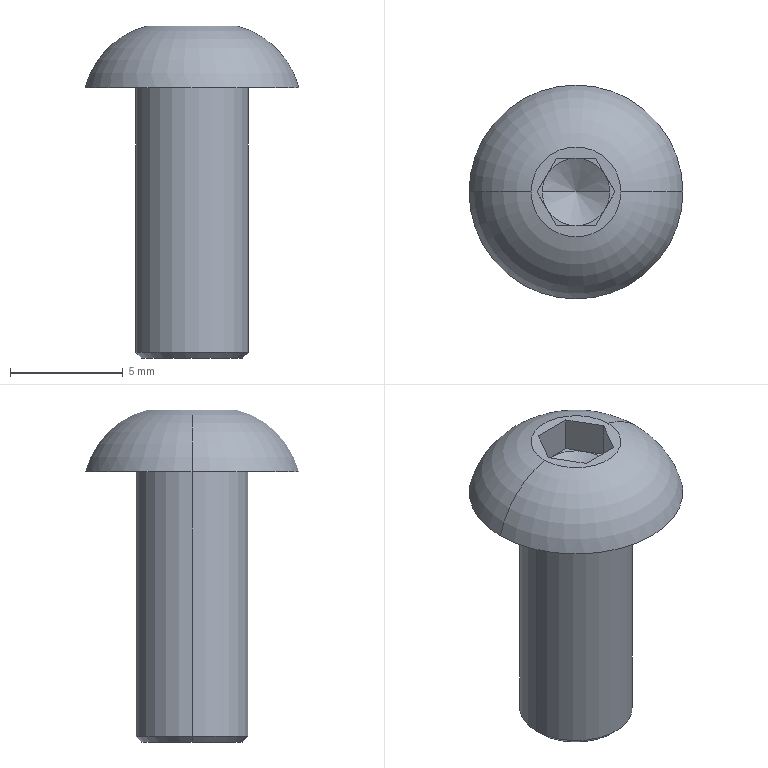Part | NX | features BREP 1 | 1 solid | 23 faces | box 9.5 x 9.5 x 14.75 mm | volume 356.014 mm3 | plane 15 | cone 4 | torus 2 | cylinder 2 | commonest cylinder face diameters 5 x2
STEP:
#1=CARTESIAN_POINT('',(0.,0.,0.324));
#2=VERTEX_POINT('',#1);
#3=CARTESIAN_POINT('',(-1.5,0.,1.19));
#4=VERTEX_POINT('',#3);
#5=CARTESIAN_POINT('',(-1.5,0.,1.19));
#6=DIRECTION('',(-0.866,0.,0.5));
#7=VECTOR('',#6,1000.);
#8=LINE('',#5,#7);
#9=EDGE_CURVE('',#2,#4,#8,.T.);
#10=ORIENTED_EDGE('',*,*,#9,.F.);
#11=CARTESIAN_POINT('',(1.5,0.,1.19));
#12=VERTEX_POINT('',#11);
#13=CARTESIAN_POINT('',(1.5,0.,1.19));
#14=DIRECTION('',(0.866,0.,0.5));
#15=VECTOR('',#14,1000.);
#16=LINE('',#13,#15);
#17=EDGE_CURVE('',#2,#12,#16,.T.);
#18=ORIENTED_EDGE('',*,*,#17,.T.);
#19=CARTESIAN_POINT('',(1.299,0.75,1.19));
#20=VERTEX_POINT('',#19);
#21=CARTESIAN_POINT('',(0.,0.,1.19));
#22=DIRECTION('',(0.,0.,1.));
#23=DIRECTION('',(1.,0.,0.));
#24=AXIS2_PLACEMENT_3D('',#21,#22,#23);
#25=CIRCLE('',#24,1.5);
#26=EDGE_CURVE('',#12,#20,#25,.T.);
#27=ORIENTED_EDGE('',*,*,#26,.T.);
#28=CARTESIAN_POINT('',(0.,1.5,1.19));
#29=VERTEX_POINT('',#28);
#30=CARTESIAN_POINT('',(0.,0.,1.19));
#31=DIRECTION('',(0.,0.,1.));
#32=DIRECTION('',(1.,0.,0.));
#33=AXIS2_PLACEMENT_3D('',#30,#31,#32);
#34=CIRCLE('',#33,1.5);
#35=EDGE_CURVE('',#20,#29,#34,.T.);
#36=ORIENTED_EDGE('',*,*,#35,.T.);
#37=CARTESIAN_POINT('',(-1.299,0.75,1.19));
#38=VERTEX_POINT('',#37);
#39=CARTESIAN_POINT('',(0.,0.,1.19));
#40=DIRECTION('',(0.,0.,-1.));
#41=DIRECTION('',(-1.,0.,0.));
#42=AXIS2_PLACEMENT_3D('',#39,#40,#41);
#43=CIRCLE('',#42,1.5);
#44=EDGE_CURVE('',#38,#29,#43,.T.);
#45=ORIENTED_EDGE('',*,*,#44,.F.);
#46=CARTESIAN_POINT('',(0.,0.,1.19));
#47=DIRECTION('',(0.,0.,1.));
#48=DIRECTION('',(1.,0.,0.));
#49=AXIS2_PLACEMENT_3D('',#46,#47,#48);
#50=CIRCLE('',#49,1.5);
#51=EDGE_CURVE('',#38,#4,#50,.T.);
#52=ORIENTED_EDGE('',*,*,#51,.T.);
#53=EDGE_LOOP('',(#10,#18,#27,#36,#45,#52));
#54=FACE_BOUND('',#53,.T.);
#55=CARTESIAN_POINT('',(0.,0.,1.19));
#56=DIRECTION('',(0.,0.,1.));
#57=DIRECTION('',(-1.,0.,0.));
#58=AXIS2_PLACEMENT_3D('',#55,#56,#57);
#59=CONICAL_SURFACE('',#58,1.5,1.047);
#60=ADVANCED_FACE('',(#54),#59,.F.);
#61=CARTESIAN_POINT('',(-2.25,0.,-12.));
#62=VERTEX_POINT('',#61);
#63=CARTESIAN_POINT('',(2.25,0.,-12.));
#64=VERTEX_POINT('',#63);
#65=CARTESIAN_POINT('',(0.,0.,-12.));
#66=DIRECTION('',(0.,0.,1.));
#67=DIRECTION('',(-1.,0.,0.));
#68=AXIS2_PLACEMENT_3D('',#65,#66,#67);
#69=CIRCLE('',#68,2.25);
#70=EDGE_CURVE('',#62,#64,#69,.T.);
#71=ORIENTED_EDGE('',*,*,#70,.T.);
#72=CARTESIAN_POINT('',(2.5,0.,-11.75));
#73=VERTEX_POINT('',#72);
#74=CARTESIAN_POINT('',(2.5,0.,-11.75));
#75=DIRECTION('',(0.7071,0.,0.7071));
#76=VECTOR('',#75,1000.);
#77=LINE('',#74,#76);
#78=EDGE_CURVE('',#64,#73,#77,.T.);
#79=ORIENTED_EDGE('',*,*,#78,.T.);
#80=CARTESIAN_POINT('',(-2.5,0.,-11.75));
#81=VERTEX_POINT('',#80);
#82=CARTESIAN_POINT('',(0.,0.,-11.75));
#83=DIRECTION('',(0.,0.,-1.));
#84=DIRECTION('',(-1.,0.,0.));
#85=AXIS2_PLACEMENT_3D('',#82,#83,#84);
#86=CIRCLE('',#85,2.5);
#87=EDGE_CURVE('',#73,#81,#86,.T.);
#88=ORIENTED_EDGE('',*,*,#87,.T.);
#89=CARTESIAN_POINT('',(-2.5,0.,-11.75));
#90=DIRECTION('',(-0.7071,0.,0.7071));
#91=VECTOR('',#90,1000.);
#92=LINE('',#89,#91);
#93=EDGE_CURVE('',#62,#81,#92,.T.);
#94=ORIENTED_EDGE('',*,*,#93,.F.);
#95=EDGE_LOOP('',(#71,#79,#88,#94));
#96=FACE_BOUND('',#95,.T.);
#97=CARTESIAN_POINT('',(0.,0.,-11.75));
#98=DIRECTION('',(0.,0.,1.));
#99=DIRECTION('',(-1.,0.,0.));
#100=AXIS2_PLACEMENT_3D('',#97,#98,#99);
#101=CONICAL_SURFACE('',#100,2.5,0.7854);
#102=ADVANCED_FACE('',(#96),#101,.T.);
#103=CARTESIAN_POINT('',(4.75,0.,0.));
#104=VERTEX_POINT('',#103);
#105=CARTESIAN_POINT('',(-4.75,0.,0.));
#106=VERTEX_POINT('',#105);
#107=CARTESIAN_POINT('',(0.,0.,0.));
#108=DIRECTION('',(0.,0.,-1.));
#109=DIRECTION('',(-1.,0.,0.));
#110=AXIS2_PLACEMENT_3D('',#107,#108,#109);
#111=CIRCLE('',#110,4.75);
#112=EDGE_CURVE('',#104,#106,#111,.T.);
#113=ORIENTED_EDGE('',*,*,#112,.F.);
#114=CARTESIAN_POINT('',(2.,0.,2.75));
#115=VERTEX_POINT('',#114);
#116=CARTESIAN_POINT('',(1.066,0.,-0.9335));
#117=DIRECTION('',(0.,-1.,0.));
#118=DIRECTION('',(1.,0.,0.));
#119=AXIS2_PLACEMENT_3D('',#116,#117,#118);
#120=CIRCLE('',#119,3.8);
#121=EDGE_CURVE('',#104,#115,#120,.T.);
#122=ORIENTED_EDGE('',*,*,#121,.T.);
#123=CARTESIAN_POINT('',(-2.,0.,2.75));
#124=VERTEX_POINT('',#123);
#125=CARTESIAN_POINT('',(0.,0.,2.75));
#126=DIRECTION('',(0.,0.,-1.));
#127=DIRECTION('',(-1.,0.,0.));
#128=AXIS2_PLACEMENT_3D('',#125,#126,#127);
#129=CIRCLE('',#128,2.);
#130=EDGE_CURVE('',#115,#124,#129,.T.);
#131=ORIENTED_EDGE('',*,*,#130,.T.);
#132=CARTESIAN_POINT('',(-1.066,0.,-0.9335));
#133=DIRECTION('',(0.,1.,0.));
#134=DIRECTION('',(0.,0.,1.));
#135=AXIS2_PLACEMENT_3D('',#132,#133,#134);
#136=CIRCLE('',#135,3.8);
#137=EDGE_CURVE('',#106,#124,#136,.T.);
#138=ORIENTED_EDGE('',*,*,#137,.F.);
#139=EDGE_LOOP('',(#113,#122,#131,#138));
#140=FACE_BOUND('',#139,.T.);
#141=CARTESIAN_POINT('',(0.,0.,-0.9335));
#142=DIRECTION('',(0.,0.,1.));
#143=DIRECTION('',(-1.,0.,0.));
#144=AXIS2_PLACEMENT_3D('',#141,#142,#143);
#145=DEGENERATE_TOROIDAL_SURFACE('',#144,1.066,3.8,.T.);
#146=ADVANCED_FACE('',(#140),#145,.T.);
#147=ORIENTED_EDGE('',*,*,#87,.F.);
#148=CARTESIAN_POINT('',(2.5,0.,0.));
#149=VERTEX_POINT('',#148);
#150=CARTESIAN_POINT('',(2.5,0.,-12.));
#151=DIRECTION('',(0.,0.,1.));
#152=VECTOR('',#151,1000.);
#153=LINE('',#150,#152);
#154=EDGE_CURVE('',#73,#149,#153,.T.);
#155=ORIENTED_EDGE('',*,*,#154,.T.);
#156=CARTESIAN_POINT('',(-2.5,0.,0.));
#157=VERTEX_POINT('',#156);
#158=CARTESIAN_POINT('',(0.,0.,0.));
#159=DIRECTION('',(0.,0.,1.));
#160=DIRECTION('',(1.,0.,0.));
#161=AXIS2_PLACEMENT_3D('',#158,#159,#160);
#162=CIRCLE('',#161,2.5);
#163=EDGE_CURVE('',#157,#149,#162,.T.);
#164=ORIENTED_EDGE('',*,*,#163,.F.);
#165=CARTESIAN_POINT('',(-2.5,0.,-12.));
#166=DIRECTION('',(0.,0.,1.));
#167=VECTOR('',#166,1000.);
#168=LINE('',#165,#167);
#169=EDGE_CURVE('',#81,#157,#168,.T.);
#170=ORIENTED_EDGE('',*,*,#169,.F.);
#171=EDGE_LOOP('',(#147,#155,#164,#170));
#172=FACE_BOUND('',#171,.T.);
#173=CARTESIAN_POINT('',(0.,0.,-12.));
#174=DIRECTION('',(0.,0.,1.));
#175=DIRECTION('',(-1.,0.,0.));
#176=AXIS2_PLACEMENT_3D('',#173,#174,#175);
#177=CYLINDRICAL_SURFACE('',#176,2.5);
#178=ADVANCED_FACE('',(#172),#177,.T.);
#179=CARTESIAN_POINT('',(0.866,1.5,1.19));
#180=VERTEX_POINT('',#179);
#181=CARTESIAN_POINT('',(1.732,0.,1.19));
#182=DIRECTION('',(-0.5,0.866,0.));
#183=VECTOR('',#182,1000.);
#184=LINE('',#181,#183);
#185=EDGE_CURVE('',#20,#180,#184,.T.);
#186=ORIENTED_EDGE('',*,*,#185,.T.);
#187=CARTESIAN_POINT('',(0.866,1.5,1.19));
#188=DIRECTION('',(-1.,0.,0.));
#189=VECTOR('',#188,1000.);
#190=LINE('',#187,#189);
#191=EDGE_CURVE('',#180,#29,#190,.T.);
#192=ORIENTED_EDGE('',*,*,#191,.T.);
#193=ORIENTED_EDGE('',*,*,#35,.F.);
#194=EDGE_LOOP('',(#186,#192,#193));
#195=FACE_BOUND('',#194,.T.);
#196=CARTESIAN_POINT('',(0.,0.,1.19));
#197=DIRECTION('',(0.,0.,-1.));
#198=DIRECTION('',(0.,-1.,0.));
#199=AXIS2_PLACEMENT_3D('',#196,#197,#198);
#200=PLANE('',#199);
#201=ADVANCED_FACE('',(#195),#200,.F.);
#202=CARTESIAN_POINT('',(-0.866,1.5,1.19));
#203=VERTEX_POINT('',#202);
#204=CARTESIAN_POINT('',(0.866,1.5,1.19));
#205=DIRECTION('',(-1.,0.,0.));
#206=VECTOR('',#205,1000.);
#207=LINE('',#204,#206);
#208=EDGE_CURVE('',#29,#203,#207,.T.);
#209=ORIENTED_EDGE('',*,*,#208,.T.);
#210=CARTESIAN_POINT('',(-0.866,1.5,1.19));
#211=DIRECTION('',(-0.5,-0.866,0.));
#212=VECTOR('',#211,1000.);
#213=LINE('',#210,#212);
#214=EDGE_CURVE('',#203,#38,#213,.T.);
#215=ORIENTED_EDGE('',*,*,#214,.T.);
#216=ORIENTED_EDGE('',*,*,#44,.T.);
#217=EDGE_LOOP('',(#209,#215,#216));
#218=FACE_BOUND('',#217,.T.);
#219=CARTESIAN_POINT('',(0.,0.,1.19));
#220=DIRECTION('',(0.,0.,-1.));
#221=DIRECTION('',(0.,-1.,0.));
#222=AXIS2_PLACEMENT_3D('',#219,#220,#221);
#223=PLANE('',#222);
#224=ADVANCED_FACE('',(#218),#223,.F.);
#225=CARTESIAN_POINT('',(-1.732,0.,1.19));
#226=VERTEX_POINT('',#225);
#227=CARTESIAN_POINT('',(-0.866,1.5,1.19));
#228=DIRECTION('',(-0.5,-0.866,0.));
#229=VECTOR('',#228,1000.);
#230=LINE('',#227,#229);
#231=EDGE_CURVE('',#38,#226,#230,.T.);
#232=ORIENTED_EDGE('',*,*,#231,.T.);
#233=CARTESIAN_POINT('',(-1.299,-0.75,1.19));
#234=VERTEX_POINT('',#233);
#235=CARTESIAN_POINT('',(-1.732,0.,1.19));
#236=DIRECTION('',(0.5,-0.866,0.));
#237=VECTOR('',#236,1000.);
#238=LINE('',#235,#237);
#239=EDGE_CURVE('',#226,#234,#238,.T.);
#240=ORIENTED_EDGE('',*,*,#239,.T.);
#241=CARTESIAN_POINT('',(0.,0.,1.19));
#242=DIRECTION('',(0.,0.,1.));
#243=DIRECTION('',(1.,0.,0.));
#244=AXIS2_PLACEMENT_3D('',#241,#242,#243);
#245=CIRCLE('',#244,1.5);
#246=EDGE_CURVE('',#4,#234,#245,.T.);
#247=ORIENTED_EDGE('',*,*,#246,.F.);
#248=ORIENTED_EDGE('',*,*,#51,.F.);
#249=EDGE_LOOP('',(#232,#240,#247,#248));
#250=FACE_BOUND('',#249,.T.);
#251=CARTESIAN_POINT('',(0.,0.,1.19));
#252=DIRECTION('',(0.,0.,-1.));
#253=DIRECTION('',(0.,-1.,0.));
#254=AXIS2_PLACEMENT_3D('',#251,#252,#253);
#255=PLANE('',#254);
#256=ADVANCED_FACE('',(#250),#255,.F.);
#257=CARTESIAN_POINT('',(-0.866,-1.5,1.19));
#258=VERTEX_POINT('',#257);
#259=CARTESIAN_POINT('',(-1.732,0.,1.19));
#260=DIRECTION('',(0.5,-0.866,0.));
#261=VECTOR('',#260,1000.);
#262=LINE('',#259,#261);
#263=EDGE_CURVE('',#234,#258,#262,.T.);
#264=ORIENTED_EDGE('',*,*,#263,.T.);
#265=CARTESIAN_POINT('',(0.,-1.5,1.19));
#266=VERTEX_POINT('',#265);
#267=CARTESIAN_POINT('',(-0.866,-1.5,1.19));
#268=DIRECTION('',(1.,0.,0.));
#269=VECTOR('',#268,1000.);
#270=LINE('',#267,#269);
#271=EDGE_CURVE('',#258,#266,#270,.T.);
#272=ORIENTED_EDGE('',*,*,#271,.T.);
#273=CARTESIAN_POINT('',(0.,0.,1.19));
#274=DIRECTION('',(0.,0.,1.));
#275=DIRECTION('',(1.,0.,0.));
#276=AXIS2_PLACEMENT_3D('',#273,#274,#275);
#277=CIRCLE('',#276,1.5);
#278=EDGE_CURVE('',#234,#266,#277,.T.);
#279=ORIENTED_EDGE('',*,*,#278,.F.);
#280=EDGE_LOOP('',(#264,#272,#279));
#281=FACE_BOUND('',#280,.T.);
#282=CARTESIAN_POINT('',(0.,0.,1.19));
#283=DIRECTION('',(0.,0.,-1.));
#284=DIRECTION('',(0.,-1.,0.));
#285=AXIS2_PLACEMENT_3D('',#282,#283,#284);
#286=PLANE('',#285);
#287=ADVANCED_FACE('',(#281),#286,.F.);
#288=CARTESIAN_POINT('',(0.866,-1.5,1.19));
#289=VERTEX_POINT('',#288);
#290=CARTESIAN_POINT('',(-0.866,-1.5,1.19));
#291=DIRECTION('',(1.,0.,0.));
#292=VECTOR('',#291,1000.);
#293=LINE('',#290,#292);
#294=EDGE_CURVE('',#266,#289,#293,.T.);
#295=ORIENTED_EDGE('',*,*,#294,.T.);
#296=CARTESIAN_POINT('',(1.299,-0.75,1.19));
#297=VERTEX_POINT('',#296);
#298=CARTESIAN_POINT('',(0.866,-1.5,1.19));
#299=DIRECTION('',(0.5,0.866,0.));
#300=VECTOR('',#299,1000.);
#301=LINE('',#298,#300);
#302=EDGE_CURVE('',#289,#297,#301,.T.);
#303=ORIENTED_EDGE('',*,*,#302,.T.);
#304=CARTESIAN_POINT('',(0.,0.,1.19));
#305=DIRECTION('',(0.,0.,1.));
#306=DIRECTION('',(1.,0.,0.));
#307=AXIS2_PLACEMENT_3D('',#304,#305,#306);
#308=CIRCLE('',#307,1.5);
#309=EDGE_CURVE('',#266,#297,#308,.T.);
#310=ORIENTED_EDGE('',*,*,#309,.F.);
#311=EDGE_LOOP('',(#295,#303,#310));
#312=FACE_BOUND('',#311,.T.);
#313=CARTESIAN_POINT('',(0.,0.,1.19));
#314=DIRECTION('',(0.,0.,-1.));
#315=DIRECTION('',(0.,-1.,0.));
#316=AXIS2_PLACEMENT_3D('',#313,#314,#315);
#317=PLANE('',#316);
#318=ADVANCED_FACE('',(#312),#317,.F.);
#319=CARTESIAN_POINT('',(0.,0.,2.75));
#320=DIRECTION('',(0.,0.,-1.));
#321=DIRECTION('',(-1.,0.,0.));
#322=AXIS2_PLACEMENT_3D('',#319,#320,#321);
#323=CIRCLE('',#322,2.);
#324=EDGE_CURVE('',#124,#115,#323,.T.);
#325=ORIENTED_EDGE('',*,*,#324,.F.);
#326=ORIENTED_EDGE('',*,*,#130,.F.);
#327=EDGE_LOOP('',(#325,#326));
#328=FACE_BOUND('',#327,.T.);
#329=CARTESIAN_POINT('',(1.732,0.,2.75));
#330=VERTEX_POINT('',#329);
#331=CARTESIAN_POINT('',(0.866,1.5,2.75));
#332=VERTEX_POINT('',#331);
#333=CARTESIAN_POINT('',(1.732,0.,2.75));
#334=DIRECTION('',(-0.5,0.866,0.));
#335=VECTOR('',#334,1000.);
#336=LINE('',#333,#335);
#337=EDGE_CURVE('',#330,#332,#336,.T.);
#338=ORIENTED_EDGE('',*,*,#337,.F.);
#339=CARTESIAN_POINT('',(0.866,-1.5,2.75));
#340=VERTEX_POINT('',#339);
#341=CARTESIAN_POINT('',(0.866,-1.5,2.75));
#342=DIRECTION('',(0.5,0.866,0.));
#343=VECTOR('',#342,1000.);
#344=LINE('',#341,#343);
#345=EDGE_CURVE('',#340,#330,#344,.T.);
#346=ORIENTED_EDGE('',*,*,#345,.F.);
#347=CARTESIAN_POINT('',(-0.866,-1.5,2.75));
#348=VERTEX_POINT('',#347);
#349=CARTESIAN_POINT('',(-0.866,-1.5,2.75));
#350=DIRECTION('',(1.,0.,0.));
#351=VECTOR('',#350,1000.);
#352=LINE('',#349,#351);
#353=EDGE_CURVE('',#348,#340,#352,.T.);
#354=ORIENTED_EDGE('',*,*,#353,.F.);
#355=CARTESIAN_POINT('',(-1.732,0.,2.75));
#356=VERTEX_POINT('',#355);
#357=CARTESIAN_POINT('',(-1.732,0.,2.75));
#358=DIRECTION('',(0.5,-0.866,0.));
#359=VECTOR('',#358,1000.);
#360=LINE('',#357,#359);
#361=EDGE_CURVE('',#356,#348,#360,.T.);
#362=ORIENTED_EDGE('',*,*,#361,.F.);
#363=CARTESIAN_POINT('',(-0.866,1.5,2.75));
#364=VERTEX_POINT('',#363);
#365=CARTESIAN_POINT('',(-0.866,1.5,2.75));
#366=DIRECTION('',(-0.5,-0.866,0.));
#367=VECTOR('',#366,1000.);
#368=LINE('',#365,#367);
#369=EDGE_CURVE('',#364,#356,#368,.T.);
#370=ORIENTED_EDGE('',*,*,#369,.F.);
#371=CARTESIAN_POINT('',(0.866,1.5,2.75));
#372=DIRECTION('',(-1.,0.,0.));
#373=VECTOR('',#372,1000.);
#374=LINE('',#371,#373);
#375=EDGE_CURVE('',#332,#364,#374,.T.);
#376=ORIENTED_EDGE('',*,*,#375,.F.);
#377=EDGE_LOOP('',(#338,#346,#354,#362,#370,#376));
#378=FACE_BOUND('',#377,.T.);
#379=CARTESIAN_POINT('',(0.,0.,2.75));
#380=DIRECTION('',(0.,0.,-1.));
#381=DIRECTION('',(0.,-1.,0.));
#382=AXIS2_PLACEMENT_3D('',#379,#380,#381);
#383=PLANE('',#382);
#384=ADVANCED_FACE('',(#328,#378),#383,.F.);
#385=CARTESIAN_POINT('',(0.,0.,0.));
#386=DIRECTION('',(0.,0.,-1.));
#387=DIRECTION('',(-1.,0.,0.));
#388=AXIS2_PLACEMENT_3D('',#385,#386,#387);
#389=CIRCLE('',#388,4.75);
#390=EDGE_CURVE('',#106,#104,#389,.T.);
#391=ORIENTED_EDGE('',*,*,#390,.T.);
#392=ORIENTED_EDGE('',*,*,#112,.T.);
#393=EDGE_LOOP('',(#391,#392));
#394=FACE_BOUND('',#393,.T.);
#395=ORIENTED_EDGE('',*,*,#163,.T.);
#396=CARTESIAN_POINT('',(0.,0.,0.));
#397=DIRECTION('',(0.,0.,1.));
#398=DIRECTION('',(1.,0.,0.));
#399=AXIS2_PLACEMENT_3D('',#396,#397,#398);
#400=CIRCLE('',#399,2.5);
#401=EDGE_CURVE('',#149,#157,#400,.T.);
#402=ORIENTED_EDGE('',*,*,#401,.T.);
#403=EDGE_LOOP('',(#395,#402));
#404=FACE_BOUND('',#403,.T.);
#405=CARTESIAN_POINT('',(0.,0.,0.));
#406=DIRECTION('',(0.,0.,-1.));
#407=DIRECTION('',(0.,-1.,0.));
#408=AXIS2_PLACEMENT_3D('',#405,#406,#407);
#409=PLANE('',#408);
#410=ADVANCED_FACE('',(#394,#404),#409,.T.);
#411=ORIENTED_EDGE('',*,*,#154,.F.);
#412=CARTESIAN_POINT('',(0.,0.,-11.75));
#413=DIRECTION('',(0.,0.,-1.));
#414=DIRECTION('',(-1.,0.,0.));
#415=AXIS2_PLACEMENT_3D('',#412,#413,#414);
#416=CIRCLE('',#415,2.5);
#417=EDGE_CURVE('',#81,#73,#416,.T.);
#418=ORIENTED_EDGE('',*,*,#417,.F.);
#419=ORIENTED_EDGE('',*,*,#169,.T.);
#420=ORIENTED_EDGE('',*,*,#401,.F.);
#421=EDGE_LOOP('',(#411,#418,#419,#420));
#422=FACE_BOUND('',#421,.T.);
#423=CARTESIAN_POINT('',(0.,0.,-12.));
#424=DIRECTION('',(0.,0.,1.));
#425=DIRECTION('',(-1.,0.,0.));
#426=AXIS2_PLACEMENT_3D('',#423,#424,#425);
#427=CYLINDRICAL_SURFACE('',#426,2.5);
#428=ADVANCED_FACE('',(#422),#427,.T.);
#429=ORIENTED_EDGE('',*,*,#70,.F.);
#430=CARTESIAN_POINT('',(0.,0.,-12.));
#431=DIRECTION('',(0.,0.,1.));
#432=DIRECTION('',(-1.,0.,0.));
#433=AXIS2_PLACEMENT_3D('',#430,#431,#432);
#434=CIRCLE('',#433,2.25);
#435=EDGE_CURVE('',#64,#62,#434,.T.);
#436=ORIENTED_EDGE('',*,*,#435,.F.);
#437=EDGE_LOOP('',(#429,#436));
#438=FACE_BOUND('',#437,.T.);
#439=CARTESIAN_POINT('',(0.,0.,-12.));
#440=DIRECTION('',(0.,0.,1.));
#441=DIRECTION('',(1.,0.,0.));
#442=AXIS2_PLACEMENT_3D('',#439,#440,#441);
#443=PLANE('',#442);
#444=ADVANCED_FACE('',(#438),#443,.F.);
#445=ORIENTED_EDGE('',*,*,#121,.F.);
#446=ORIENTED_EDGE('',*,*,#390,.F.);
#447=ORIENTED_EDGE('',*,*,#137,.T.);
#448=ORIENTED_EDGE('',*,*,#324,.T.);
#449=EDGE_LOOP('',(#445,#446,#447,#448));
#450=FACE_BOUND('',#449,.T.);
#451=CARTESIAN_POINT('',(0.,0.,-0.9335));
#452=DIRECTION('',(0.,0.,1.));
#453=DIRECTION('',(-1.,0.,0.));
#454=AXIS2_PLACEMENT_3D('',#451,#452,#453);
#455=DEGENERATE_TOROIDAL_SURFACE('',#454,1.066,3.8,.T.);
#456=ADVANCED_FACE('',(#450),#455,.T.);
#457=ORIENTED_EDGE('',*,*,#78,.F.);
#458=ORIENTED_EDGE('',*,*,#435,.T.);
#459=ORIENTED_EDGE('',*,*,#93,.T.);
#460=ORIENTED_EDGE('',*,*,#417,.T.);
#461=EDGE_LOOP('',(#457,#458,#459,#460));
#462=FACE_BOUND('',#461,.T.);
#463=CARTESIAN_POINT('',(0.,0.,-11.75));
#464=DIRECTION('',(0.,0.,1.));
#465=DIRECTION('',(-1.,0.,0.));
#466=AXIS2_PLACEMENT_3D('',#463,#464,#465);
#467=CONICAL_SURFACE('',#466,2.5,0.7854);
#468=ADVANCED_FACE('',(#462),#467,.T.);
#469=ORIENTED_EDGE('',*,*,#337,.T.);
#470=CARTESIAN_POINT('',(0.866,1.5,1.19));
#471=DIRECTION('',(0.,0.,1.));
#472=VECTOR('',#471,1000.);
#473=LINE('',#470,#472);
#474=EDGE_CURVE('',#180,#332,#473,.T.);
#475=ORIENTED_EDGE('',*,*,#474,.F.);
#476=ORIENTED_EDGE('',*,*,#185,.F.);
#477=CARTESIAN_POINT('',(1.732,0.,1.19));
#478=VERTEX_POINT('',#477);
#479=CARTESIAN_POINT('',(1.732,0.,1.19));
#480=DIRECTION('',(-0.5,0.866,0.));
#481=VECTOR('',#480,1000.);
#482=LINE('',#479,#481);
#483=EDGE_CURVE('',#478,#20,#482,.T.);
#484=ORIENTED_EDGE('',*,*,#483,.F.);
#485=CARTESIAN_POINT('',(1.732,0.,1.19));
#486=DIRECTION('',(0.,0.,1.));
#487=VECTOR('',#486,1000.);
#488=LINE('',#485,#487);
#489=EDGE_CURVE('',#478,#330,#488,.T.);
#490=ORIENTED_EDGE('',*,*,#489,.T.);
#491=EDGE_LOOP('',(#469,#475,#476,#484,#490));
#492=FACE_BOUND('',#491,.T.);
#493=CARTESIAN_POINT('',(1.732,0.,1.19));
#494=DIRECTION('',(-0.866,-0.5,0.));
#495=DIRECTION('',(-0.5,0.866,0.));
#496=AXIS2_PLACEMENT_3D('',#493,#494,#495);
#497=PLANE('',#496);
#498=ADVANCED_FACE('',(#492),#497,.T.);
#499=ORIENTED_EDGE('',*,*,#375,.T.);
#500=CARTESIAN_POINT('',(-0.866,1.5,1.19));
#501=DIRECTION('',(0.,0.,1.));
#502=VECTOR('',#501,1000.);
#503=LINE('',#500,#502);
#504=EDGE_CURVE('',#203,#364,#503,.T.);
#505=ORIENTED_EDGE('',*,*,#504,.F.);
#506=ORIENTED_EDGE('',*,*,#208,.F.);
#507=ORIENTED_EDGE('',*,*,#191,.F.);
#508=ORIENTED_EDGE('',*,*,#474,.T.);
#509=EDGE_LOOP('',(#499,#505,#506,#507,#508));
#510=FACE_BOUND('',#509,.T.);
#511=CARTESIAN_POINT('',(0.866,1.5,1.19));
#512=DIRECTION('',(0.,-1.,0.));
#513=DIRECTION('',(0.,0.,-1.));
#514=AXIS2_PLACEMENT_3D('',#511,#512,#513);
#515=PLANE('',#514);
#516=ADVANCED_FACE('',(#510),#515,.T.);
#517=ORIENTED_EDGE('',*,*,#369,.T.);
#518=CARTESIAN_POINT('',(-1.732,0.,1.19));
#519=DIRECTION('',(0.,0.,1.));
#520=VECTOR('',#519,1000.);
#521=LINE('',#518,#520);
#522=EDGE_CURVE('',#226,#356,#521,.T.);
#523=ORIENTED_EDGE('',*,*,#522,.F.);
#524=ORIENTED_EDGE('',*,*,#231,.F.);
#525=ORIENTED_EDGE('',*,*,#214,.F.);
#526=ORIENTED_EDGE('',*,*,#504,.T.);
#527=EDGE_LOOP('',(#517,#523,#524,#525,#526));
#528=FACE_BOUND('',#527,.T.);
#529=CARTESIAN_POINT('',(-0.866,1.5,1.19));
#530=DIRECTION('',(0.866,-0.5,0.));
#531=DIRECTION('',(0.,0.,-1.));
#532=AXIS2_PLACEMENT_3D('',#529,#530,#531);
#533=PLANE('',#532);
#534=ADVANCED_FACE('',(#528),#533,.T.);
#535=ORIENTED_EDGE('',*,*,#361,.T.);
#536=CARTESIAN_POINT('',(-0.866,-1.5,1.19));
#537=DIRECTION('',(0.,0.,1.));
#538=VECTOR('',#537,1000.);
#539=LINE('',#536,#538);
#540=EDGE_CURVE('',#258,#348,#539,.T.);
#541=ORIENTED_EDGE('',*,*,#540,.F.);
#542=ORIENTED_EDGE('',*,*,#263,.F.);
#543=ORIENTED_EDGE('',*,*,#239,.F.);
#544=ORIENTED_EDGE('',*,*,#522,.T.);
#545=EDGE_LOOP('',(#535,#541,#542,#543,#544));
#546=FACE_BOUND('',#545,.T.);
#547=CARTESIAN_POINT('',(-1.732,0.,1.19));
#548=DIRECTION('',(0.866,0.5,0.));
#549=DIRECTION('',(0.,0.,-1.));
#550=AXIS2_PLACEMENT_3D('',#547,#548,#549);
#551=PLANE('',#550);
#552=ADVANCED_FACE('',(#546),#551,.T.);
#553=ORIENTED_EDGE('',*,*,#353,.T.);
#554=CARTESIAN_POINT('',(0.866,-1.5,1.19));
#555=DIRECTION('',(0.,0.,1.));
#556=VECTOR('',#555,1000.);
#557=LINE('',#554,#556);
#558=EDGE_CURVE('',#289,#340,#557,.T.);
#559=ORIENTED_EDGE('',*,*,#558,.F.);
#560=ORIENTED_EDGE('',*,*,#294,.F.);
#561=ORIENTED_EDGE('',*,*,#271,.F.);
#562=ORIENTED_EDGE('',*,*,#540,.T.);
#563=EDGE_LOOP('',(#553,#559,#560,#561,#562));
#564=FACE_BOUND('',#563,.T.);
#565=CARTESIAN_POINT('',(-0.866,-1.5,1.19));
#566=DIRECTION('',(0.,1.,0.));
#567=DIRECTION('',(1.,0.,0.));
#568=AXIS2_PLACEMENT_3D('',#565,#566,#567);
#569=PLANE('',#568);
#570=ADVANCED_FACE('',(#564),#569,.T.);
#571=ORIENTED_EDGE('',*,*,#345,.T.);
#572=ORIENTED_EDGE('',*,*,#489,.F.);
#573=CARTESIAN_POINT('',(0.866,-1.5,1.19));
#574=DIRECTION('',(0.5,0.866,0.));
#575=VECTOR('',#574,1000.);
#576=LINE('',#573,#575);
#577=EDGE_CURVE('',#297,#478,#576,.T.);
#578=ORIENTED_EDGE('',*,*,#577,.F.);
#579=ORIENTED_EDGE('',*,*,#302,.F.);
#580=ORIENTED_EDGE('',*,*,#558,.T.);
#581=EDGE_LOOP('',(#571,#572,#578,#579,#580));
#582=FACE_BOUND('',#581,.T.);
#583=CARTESIAN_POINT('',(0.866,-1.5,1.19));
#584=DIRECTION('',(-0.866,0.5,0.));
#585=DIRECTION('',(0.,0.,1.));
#586=AXIS2_PLACEMENT_3D('',#583,#584,#585);
#587=PLANE('',#586);
#588=ADVANCED_FACE('',(#582),#587,.T.);
#589=ORIENTED_EDGE('',*,*,#577,.T.);
#590=ORIENTED_EDGE('',*,*,#483,.T.);
#591=ORIENTED_EDGE('',*,*,#26,.F.);
#592=CARTESIAN_POINT('',(0.,0.,1.19));
#593=DIRECTION('',(0.,0.,1.));
#594=DIRECTION('',(1.,0.,0.));
#595=AXIS2_PLACEMENT_3D('',#592,#593,#594);
#596=CIRCLE('',#595,1.5);
#597=EDGE_CURVE('',#297,#12,#596,.T.);
#598=ORIENTED_EDGE('',*,*,#597,.F.);
#599=EDGE_LOOP('',(#589,#590,#591,#598));
#600=FACE_BOUND('',#599,.T.);
#601=CARTESIAN_POINT('',(0.,0.,1.19));
#602=DIRECTION('',(0.,0.,-1.));
#603=DIRECTION('',(0.,-1.,0.));
#604=AXIS2_PLACEMENT_3D('',#601,#602,#603);
#605=PLANE('',#604);
#606=ADVANCED_FACE('',(#600),#605,.F.);
#607=ORIENTED_EDGE('',*,*,#17,.F.);
#608=ORIENTED_EDGE('',*,*,#9,.T.);
#609=ORIENTED_EDGE('',*,*,#246,.T.);
#610=ORIENTED_EDGE('',*,*,#278,.T.);
#611=ORIENTED_EDGE('',*,*,#309,.T.);
#612=ORIENTED_EDGE('',*,*,#597,.T.);
#613=EDGE_LOOP('',(#607,#608,#609,#610,#611,#612));
#614=FACE_BOUND('',#613,.T.);
#615=CARTESIAN_POINT('',(0.,0.,1.19));
#616=DIRECTION('',(0.,0.,1.));
#617=DIRECTION('',(-1.,0.,0.));
#618=AXIS2_PLACEMENT_3D('',#615,#616,#617);
#619=CONICAL_SURFACE('',#618,1.5,1.047);
#620=ADVANCED_FACE('',(#614),#619,.F.);
#621=CLOSED_SHELL('',(#60,#102,#146,#178,#201,#224,#256,#287,#318,#384,#410,#428,#444,#456,#468,#498,#516,#534,#552,#570,#588,#606,#620));
#622=MANIFOLD_SOLID_BREP('',#621);
#623=(LENGTH_UNIT()NAMED_UNIT(*)SI_UNIT(.MILLI.,.METRE.));
#624=UNCERTAINTY_MEASURE_WITH_UNIT(LENGTH_MEASURE(0.00001),#623,'','');
#625=(NAMED_UNIT(*)PLANE_ANGLE_UNIT()SI_UNIT($,.RADIAN.));
#626=(NAMED_UNIT(*)SI_UNIT($,.STERADIAN.)SOLID_ANGLE_UNIT());
#627=(GEOMETRIC_REPRESENTATION_CONTEXT(3)GLOBAL_UNCERTAINTY_ASSIGNED_CONTEXT((#624))GLOBAL_UNIT_ASSIGNED_CONTEXT((#623,#625,#626))REPRESENTATION_CONTEXT('',''));
#628=ADVANCED_BREP_SHAPE_REPRESENTATION('',(#622),#627);